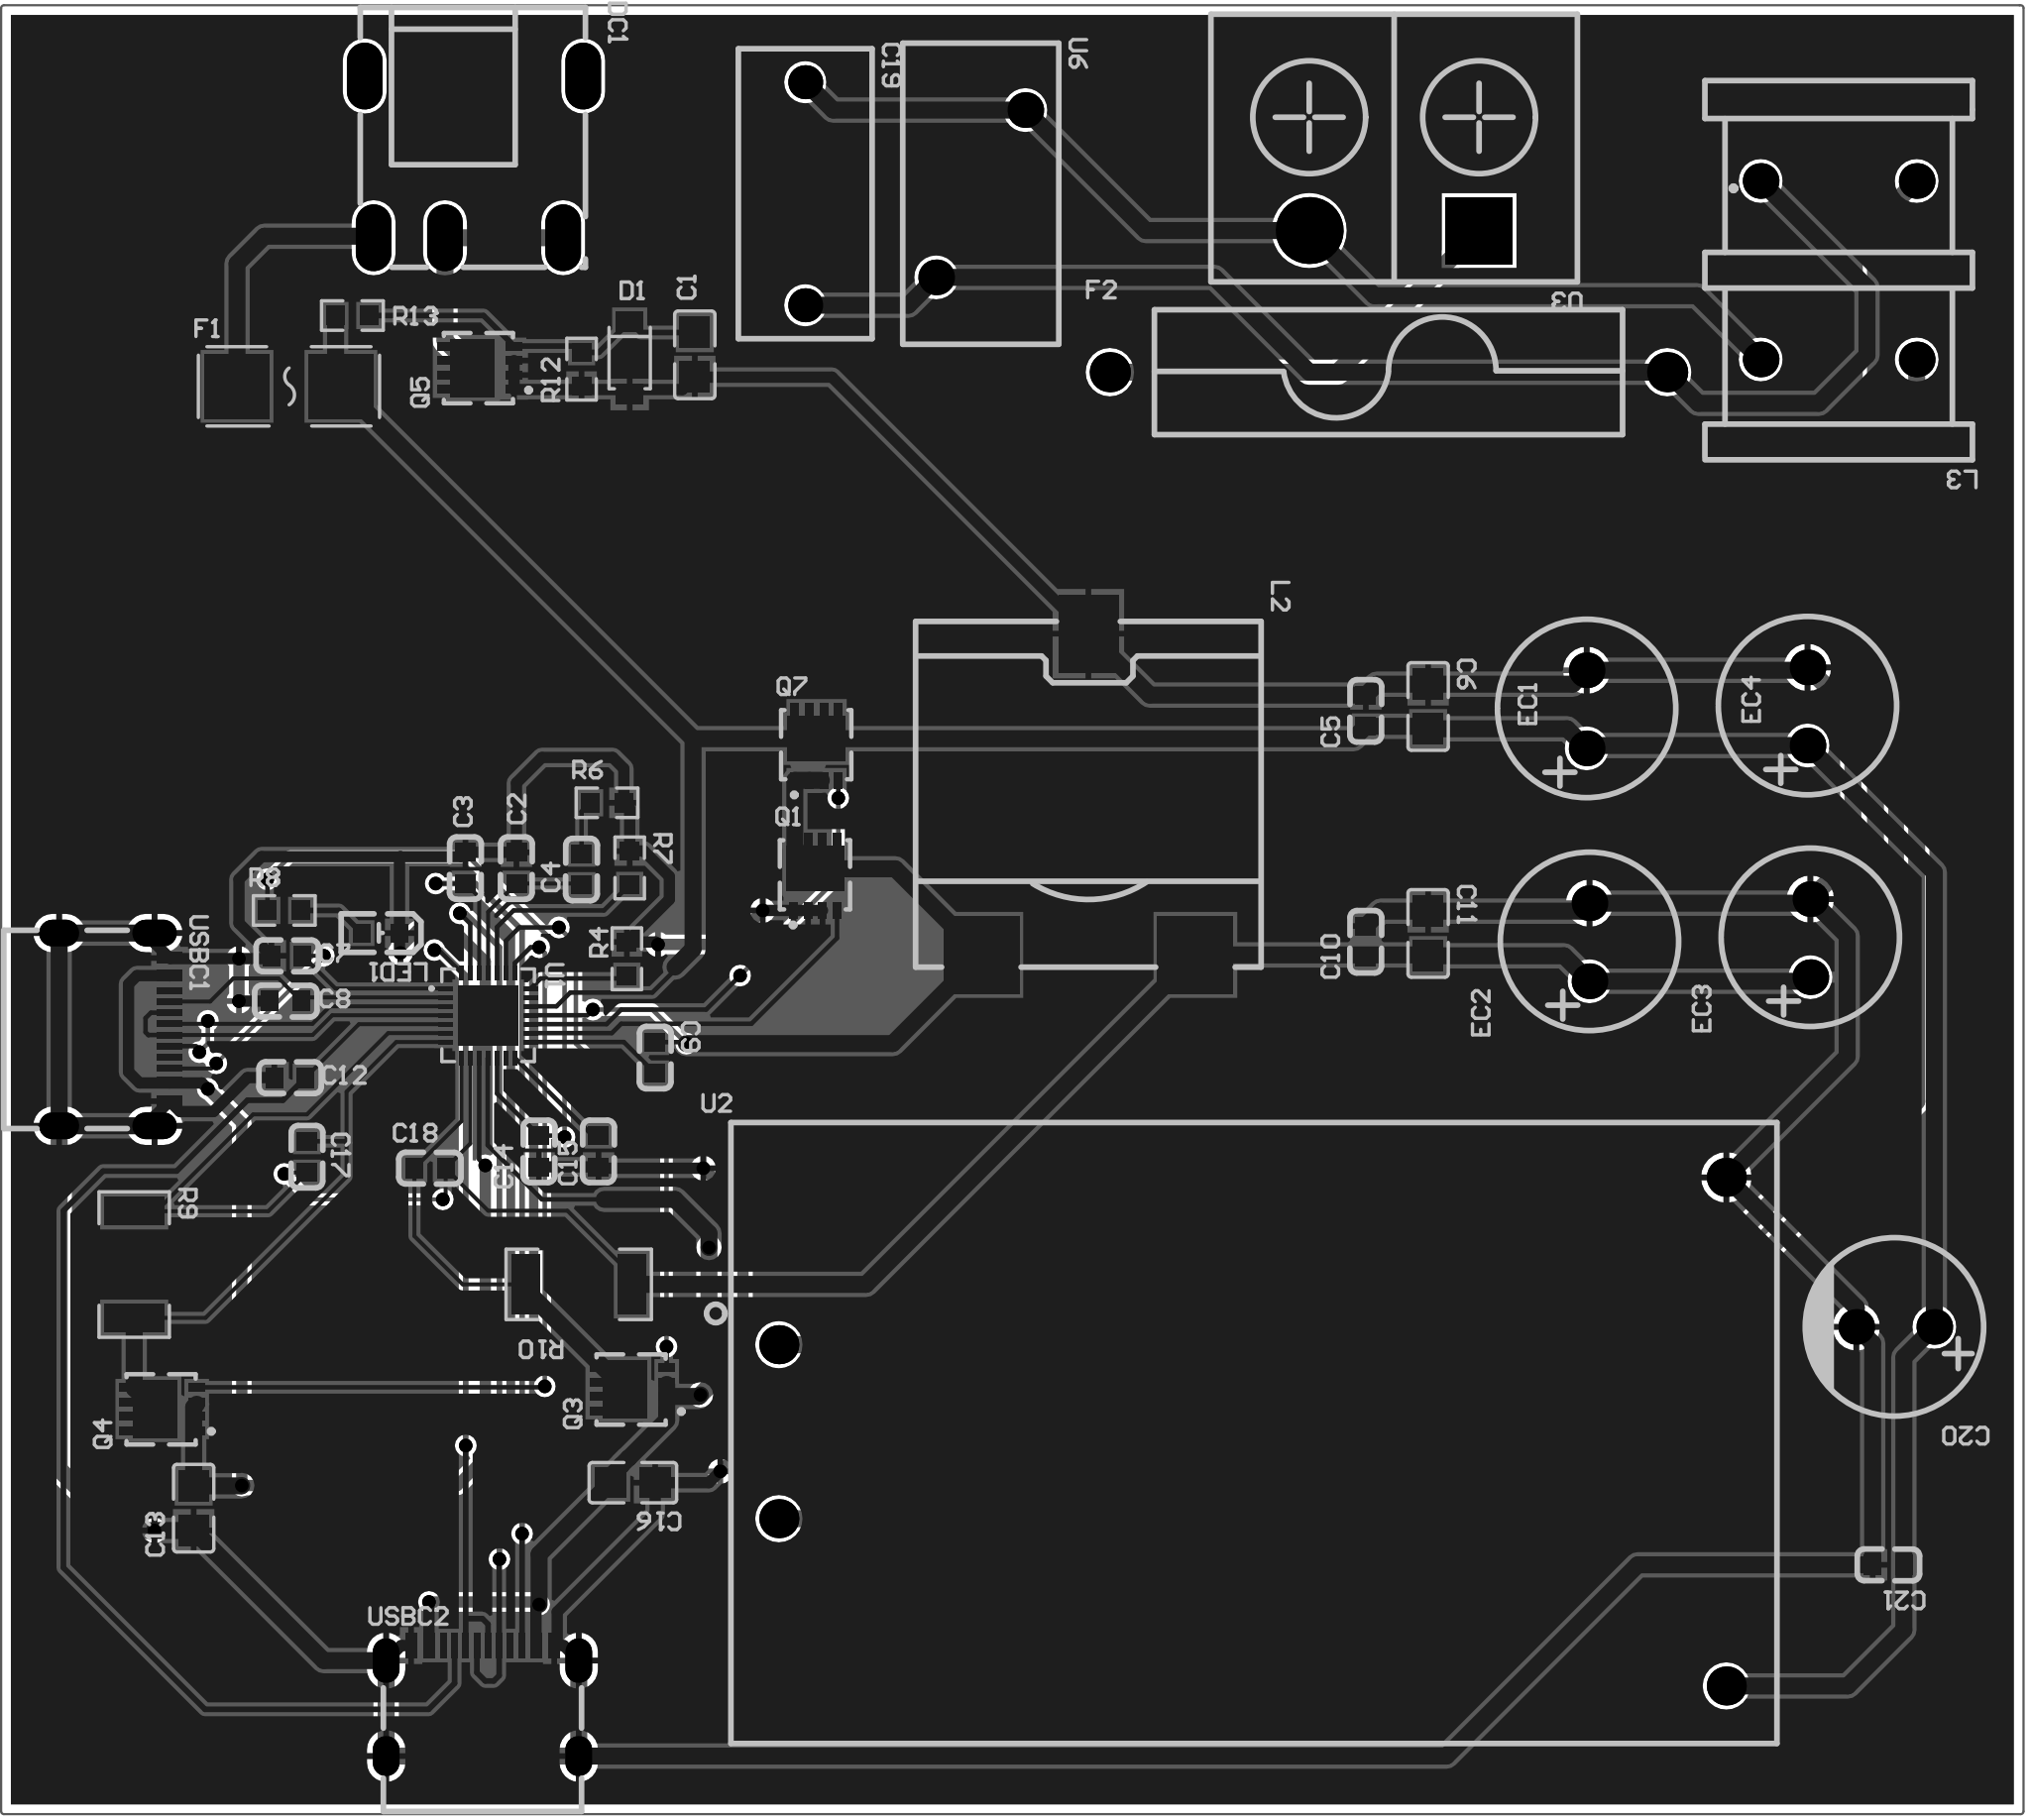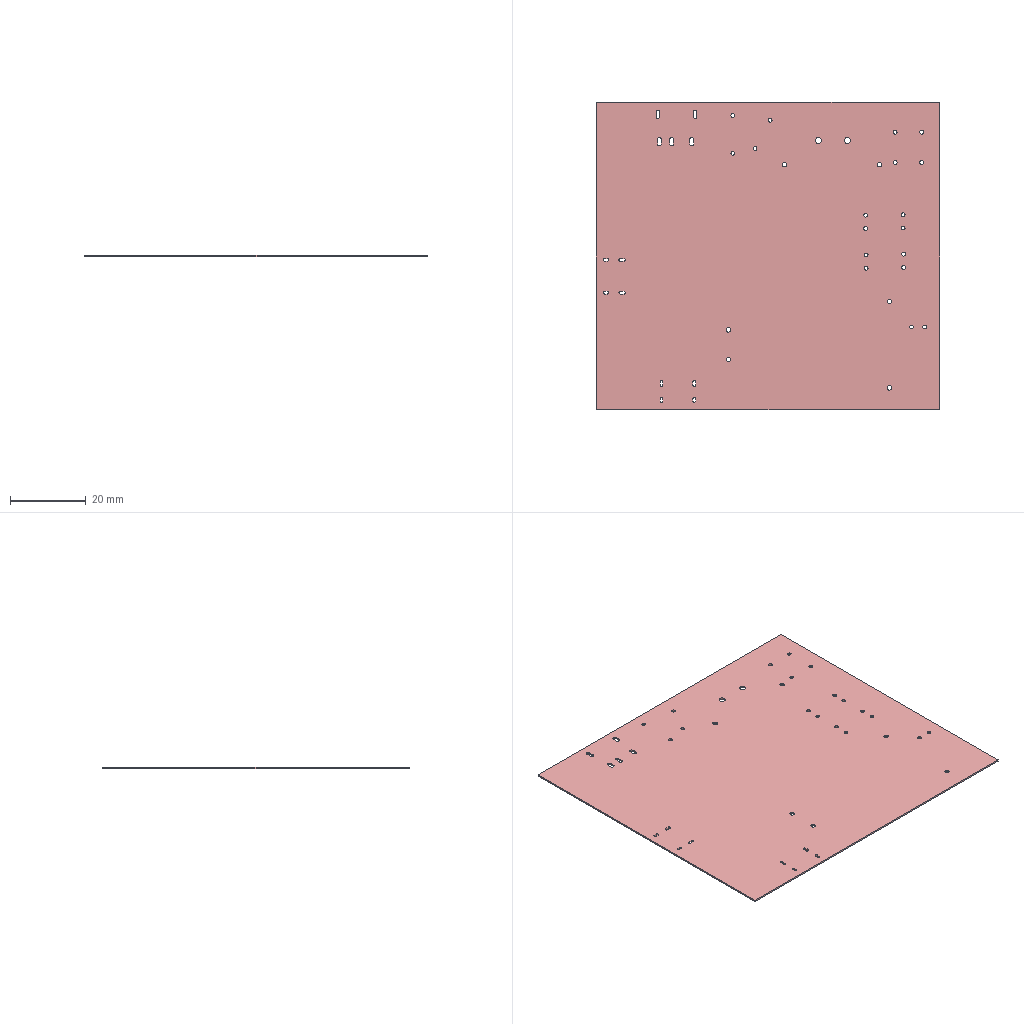Circuit board layout | Altium Designer | box 90.7 x 81.1 x 0.4 mm
Layer stack:
# Altium Designer layer stack of  (unit mm; dielectric type: 0 none, 1 core, 2 prepreg, 3 surface material)
index,name,kind,layer,copper_thickness_mm,dielectric_type,dielectric_thickness_mm,dielectric_material,dielectric_constant
0,Top Solder Mask Layer,dielectric,,,3,0.0102,Solder Resist,3.5
1,Top Paste Mask Layer,other,,,,,,
2,Top Silkscreen Layer,other,,,,,,
3,Top Layer,copper,Top Layer,0.0356,,,,
4,Dielectric1,dielectric,,,0,0.32,FR-4,4.8
5,Bottom Layer,copper,Bottom Layer,0.0356,,,,
6,Bottom Silkscreen Layer,other,,,,,,
7,Bottom Paste Mask Layer,other,,,,,,
8,Bottom Solder Mask Layer,dielectric,,,3,0.0102,Solder Resist,3.5
# drill layer pairs: low layer,high layer
drill_pair,Top Layer,Bottom Layer
Part placement:
Designator,Comment,Layer,Footprint,Center-X(mm),Center-Y(mm),Rotation
C21,100nF,TopLayer,C0603,154.37,80.899,180
C20,220uF,TopLayer,CAP-TH_BD8.0-P3.50-D0.6-FD,154.686,91.567,180
F2,5G0.001522S1(5),TopLayer,FUSE-TH_BD5.6-L21.0-P25.00-D0.7,131.953,134.366,360
L3,UU9.8-20mH,TopLayer,FILTER-TH_4P-L17.0-W12.0-P7.00-D0.6-S8.00,152.146,138.938,180
C19,100nF,TopLayer,CAP-TH_L13.0-W6.0-P10.0-D0.6,105.791,142.367,270
U6,10D561K68RV0095,TopLayer,RES-TH_L13.5-W7.0-P7.50-S4.00-D0.7,113.665,142.367,270
U3,KF7.62-2P,TopLayer,CONN-TH_KF7.62-2P,132.207,140.716,180
U2,HLK-10M24,TopLayer,PWRM-TH_HLK-10M24,125.857,86.868,360
R4,Rpset,TopLayer,R0603,97.79,108.068,270
LED1,19-217/BHC-ZL1M2RY/3T,TopLayer,LED0603-R-RD,86.741,109.22,180
R13,0603WAF5102T5E,TopLayer,R0603,85.48,136.906,180
U1,sw3556-1,TopLayer,QFN-28_L4.0-W4.0-P0.40-BL-EP,91.567,105.537,270
C16,10uF,TopLayer,C0805,98.06,84.582,180
C13,10uF,TopLayer,C0805,78.359,83.439,90
C11,22uF,TopLayer,C0805,133.731,109.204,270
C10,100nF,TopLayer,C0603,130.937,108.839,90
C6,10uF,TopLayer,C0805,133.731,119.38,270
C5,100nF,TopLayer,C0603,130.937,119.191,90
C1,10uF,TopLayer,C0805,100.838,135.144,90
R12,10kΩ,TopLayer,R0603,95.758,134.502,90
C9,100nF,TopLayer,C0603,99.06,103.632,270
C15,1uF,TopLayer,C0603,96.52,99.441,90
C14,1uF,TopLayer,C0603,93.853,99.441,90
C18,100nF,TopLayer,C0603,88.962,98.679,360
C17,100nF,TopLayer,C0603,83.439,99.187,270
C12,330pF,TopLayer,C0603,82.677,102.743,180
C8,330pF,TopLayer,C0603,82.485,106.172,180
C7,330pF,TopLayer,C0603,82.55,108.204,180
R8,0603WAF2001T5E,TopLayer,R0603,82.423,110.236,0
R7,SDNT1608X104F4250FTF,TopLayer,R0603,97.917,112.141,270
R6,20kΩ,TopLayer,R0603,96.901,115.062,360
C4,2.2nF,TopLayer,C0603,95.758,112.076,90
C2,100pF,TopLayer,C0603,92.837,112.141,90
C3,330pF,TopLayer,C0603,90.551,112.141,90
Q5,RUH4040M2,TopLayer,PDFN3333-8_L3.1-W3.2-P0.65-LS3.4-BL,91.195,134.564,90
Q3,RUH4040M2,TopLayer,PDFN3333-8_L3.1-W3.2-P0.65-LS3.4-BL,98.044,88.773,90
Q4,RUH4040M2,TopLayer,PDFN3333-8_L3.1-W3.2-P0.65-LS3.4-BL,76.962,87.884,90
Q1,RUH4040M2,TopLayer,PDFN3333-8_L3.1-W3.2-P0.65-LS3.4-BL,106.243,111.769,360
Q7,RUH4040M2,TopLayer,PDFN3333-8_L3.1-W3.2-P0.65-LS3.4-BL,106.299,117.602,360
USBC2,U263-163N-4OS1735,TopLayer,USB-C-SMD_U263-163N-4GS1735,91.313,74.803,360
USBC1,U263-163N-4OS1735,TopLayer,USB-C-SMD_U263-163N-4GS1735,74.803,104.902,270
EC4,220uF,TopLayer,CAP-TH_BD8.0-P3.50-D0.6-FD-2,150.749,119.38,90
D1,BZT52C3V3,TopLayer,SOD-123_L2.7-W1.6-LS3.7-RD,97.917,135.001,270
F1,0451008.MRL,TopLayer,FUSE-SMD_L6.1-W2.7,82.634,133.731,0
DC1,DC-044A-20A,TopLayer,DC-IN-TH_DC-044A-20A,90.932,144.018,270
EC3,220uF,TopLayer,CAP-TH_BD8.0-P3.50-D0.6-FD-2,150.876,108.994,90
R10,RLM20FECR005,TopLayer,R2010,95.631,93.472,180
R9,RLM20FECR005,TopLayer,R2010,75.692,94.361,270
L2,22uH,TopLayer,IND-SMD_3P-L15.5-W15.5-L,118.491,115.443,270
EC2,220uF,TopLayer,CAP-TH_BD8.0-P3.50-D0.6-FD-2,140.97,108.811,90
EC1,220uF,TopLayer,CAP-TH_BD8.0-P3.50-D0.6-FD-2,140.843,119.253,90
Pad and via stacks:
# Altium Designer via and pad stacks of  (unit mm). Each distinct definition once, with the count of objects using it.
# via: kind,start_layer,end_layer,hole_mm,diameter_mm,mode(0 simple;1 top-mid-bottom;2 full stack),diameter_per_layer,count,example_net
# pad: kind,layer,hole_mm,hole_type(0 round;1 square;2 slot),plating,top_size,top_shape(1 round;2 rect;3 octagon;9 rounded rect),mid_size,bottom_size,mode,footprint,size_per_layer,count,example
pad,Multi-Layer,1,0,plated,1.6x1.6,1,1.6x1.6,1.6x1.6,0,CAP-TH_BD8.0-P3.50-D0.6-FD,,2,C20.1
pad,Multi-Layer,1.2,0,plated,1.8x1.8,1,1.8x1.8,1.8x1.8,0,FUSE-TH_BD5.6-L21.0-P25.00-D0.7,,2,F2.2
pad,Multi-Layer,1,0,plated,1.6x1.6,1,1.6x1.6,1.6x1.6,0,FILTER-TH_4P-L17.0-W12.0-P7.00-D0.6-S8.00,,4,L3.1
pad,Multi-Layer,1,0,plated,1.524x1.524,1,1.524x1.524,1.524x1.524,0,CAP-TH_L13.0-W6.0-P10.0-D0.6,,2,C19.2
pad,Multi-Layer,1,0,plated,1.6x1.6,1,1.6x1.6,1.6x1.6,0,RES-TH_L13.5-W7.0-P7.50-S4.00-D0.7,,2,U6.2
pad,Multi-Layer,1.6,0,plated,3x3,2,3x3,3x3,0,CONN-TH_KF7.62-2P,,1,U3.1
pad,Multi-Layer,1.6,0,plated,3x3,1,3x3,3x3,0,CONN-TH_KF7.62-2P,,1,U3.2
pad,Multi-Layer,1.2,0,plated,1.75x1.75,1,1.75x1.75,1.75x1.75,0,PWRM-TH_HLK-10M24,,4,U2.3
pad,Multi-Layer,0.7,2,plated,1.2x2,1,1.2x2,1.2x2,0,USB-C-SMD_U263-163N-4GS1735,,4,USBC2.SH1
pad,Multi-Layer,0.7,2,plated,1.2x1.8,1,1.2x1.8,1.2x1.8,0,USB-C-SMD_U263-163N-4GS1735,,4,USBC2.SH1
pad,Multi-Layer,1,0,plated,1.6x1.6,1,1.6x1.6,1.6x1.6,0,CAP-TH_BD8.0-P3.50-D0.6-FD-2,,8,EC4.2
pad,Multi-Layer,1,2,plated,1.6x3,1,1.6x3,1.6x3,0,DC-IN-TH_DC-044A-20A,,5,DC1.5
pad,Top Layer,0,0,plated,0.8x0.9,2,0.8x0.9,0.8x0.9,0,C0603,,28,C21.1
pad,Top Layer,0,0,plated,0.8065x0.864,2,0.8065x0.864,0.8065x0.864,0,R0603,,12,R4.1
pad,Top Layer,0,0,plated,0.8x0.8,2,0.8x0.8,0.8x0.8,0,LED0603-R-RD,,2,LED1.2
pad,Top Layer,0,0,plated,2.7x2.7,2,2.7x2.7,2.7x2.7,0,QFN-28_L4.0-W4.0-P0.40-BL-EP,,1,U1.29
pad,Top Layer,0,0,plated,0.665x0.2,2,0.665x0.2,0.665x0.2,0,QFN-28_L4.0-W4.0-P0.40-BL-EP,,14,U1.28
pad,Top Layer,0,0,plated,0.2x0.665,2,0.2x0.665,0.2x0.665,0,QFN-28_L4.0-W4.0-P0.40-BL-EP,,14,U1.21
pad,Top Layer,0,0,plated,1.41x1.35,2,1.41x1.35,1.41x1.35,0,C0805,,10,C16.1
pad,Top Layer,0,0,plated,2.6x2,2,2.6x2,2.6x2,0,PDFN3333-8_L3.1-W3.2-P0.65-LS3.4-BL,,5,Q5.9
pad,Top Layer,0,0,plated,0.4x0.8,2,0.4x0.8,0.4x0.8,0,PDFN3333-8_L3.1-W3.2-P0.65-LS3.4-BL,,20,Q5.5
pad,Top Layer,0,0,plated,0.4x0.75,2,0.4x0.75,0.4x0.75,0,PDFN3333-8_L3.1-W3.2-P0.65-LS3.4-BL,,20,Q5.4
pad,Top Layer,0,0,plated,0.5x1.15,2,0.5x1.15,0.5x1.15,0,USB-C-SMD_U263-163N-4GS1735,,16,USBC2.B1
pad,Top Layer,0,0,plated,0.3x1.15,2,0.3x1.15,0.3x1.15,0,USB-C-SMD_U263-163N-4GS1735,,16,USBC2.B5
pad,Top Layer,0,0,plated,0.91x1.22,2,0.91x1.22,0.91x1.22,0,SOD-123_L2.7-W1.6-LS3.7-RD,,2,D1.1
pad,Top Layer,0,0,plated,2.911x2.906,2,2.911x2.906,2.911x2.906,0,FUSE-SMD_L6.1-W2.7,,2,F1.1
pad,Top Layer,0,0,plated,1.282x2.7,2,1.282x2.7,1.282x2.7,0,R2010,,4,R10.1
pad,Top Layer,0,0,plated,3.5x3.401,2,3.5x3.401,3.5x3.401,0,IND-SMD_3P-L15.5-W15.5-L,,2,L2.3
pad,Top Layer,0,0,plated,3.5x2.7,2,3.5x2.7,3.5x2.7,0,IND-SMD_3P-L15.5-W15.5-L,,1,L2.1
via,Top Layer,Bottom Layer,0.3048,0.6096,0,,39,GND
Copper pours:
name,layer,net,type(0 solid;1 hatched;2 none)
Top Layer-No Net,Top Layer,GND,0
Top Layer-No Net,Bottom Layer,GND,0
Design rules, without the lines most boards share:
# Altium Designer design rules of  (exported by Altium Designer, unit mm)
# columns: name | kind | enabled | priority | scope1 | scope2 | descriptor | typed fields (field=value)
SilkToSilkClearance | 55 | enabled | 1 | All | All | Silk to Silk (Clearance=0mil) (All),(All) |
SilkToSolderMaskClearance | 54 | enabled | 1 | IsPad | All | Silk To Solder Mask (Clearance=0mil) (IsPad),(All) |
MinimumSolderMaskSliver | 53 | enabled | 1 | All | All | Minimum Solder Mask Sliver (Gap=0mil) (All),(All) |
HoleToHoleClearance | 52 | enabled | 1 | All | All | Hole To Hole Clearance (Gap=10mil) (All),(All) | gap=0.254
DiffPairsRouting | 51 | enabled | 1 | All | All | Differential Pairs Uncoupled Length using the Gap Constraints (Min=10mil) (Max=10mil) (Prefered=10mil)  and Width Constraints (Min=15mil) (Max=15mil) (Prefered=15mil) (All) |
SolderMaskExpansion | 13 | enabled | 1 | All | All | Solder Mask Expansion (Expansion =4mil) (All) | expansion=0.1016
RoutingVias | 11 | enabled | 1 | All | All | Routing Via (MinHoleWidth=28mil) (MaxHoleWidth=28mil) (PreferredHoleWidth=28mil) (MinWidth=50mil) (MaxWidth=50mil) (PreferedWidth=50mil) (All) | via_min_hole=0.7112 via_max_hole=0.7112 via_preferred_diameter=1.27 via_preferred_hole=0.7112
Width | 2 | enabled | 1 | All | All | Width Constraint (Min=7mil) (Max=50mil) (Preferred=10mil) (All) |
PolygonConnect | 20 | enabled | 1 | All | All | Polygon Connect Rule(Relief Connect )(Conductor Width=10mil) (Relief Angle=90 Angle) (Entries=4) (Air Gap Width=10mil) (All),(All) | connect_style(0=relief,1=direct,2=none)=0 relief_conductor_width=0.254 relief_entries=4
PlaneConnect | 6 | enabled | 1 | All | All | Power Plane Connect Rule(Relief Connect )(Expansion=20mil) (Conductor Width=10mil) (Air Gap=10mil) (Entries=4) (All) | relief_conductor_width=0.254 relief_entries=4 relief_expansion=0.508
Clearance | 0 | enabled | 1 | All | All | Clearance Constraint (Gap=7mil) (All),(All) | gap=0.1778
Classes set for this board:
# Altium Designer classes of  (member kind: 0 net, 1 component, 2 from-to, 3 pad, 4 layer, 5 differential pair, 6 design channel, 7 polygon, 8 structure, 9 xSignal)
# columns: class name | member kind | superclass | members
1_1_P1.schdoc.schdoc | 1 | no | C1; C2; C3; C4; C5; C6; C7; C8; C9; C10; C11; C12; C13; C14; C15; C16; C17; C18; C19; C20; C21; D1; DC1; EC1; EC2; EC3; EC4; F1; F2; L2; L3; LED1; Q1; Q3; Q4; Q5; Q7; R4; R6; R7; R8; R9; R10; R12; R13; U1; U2; U3; U6; USBC1; USBC2;